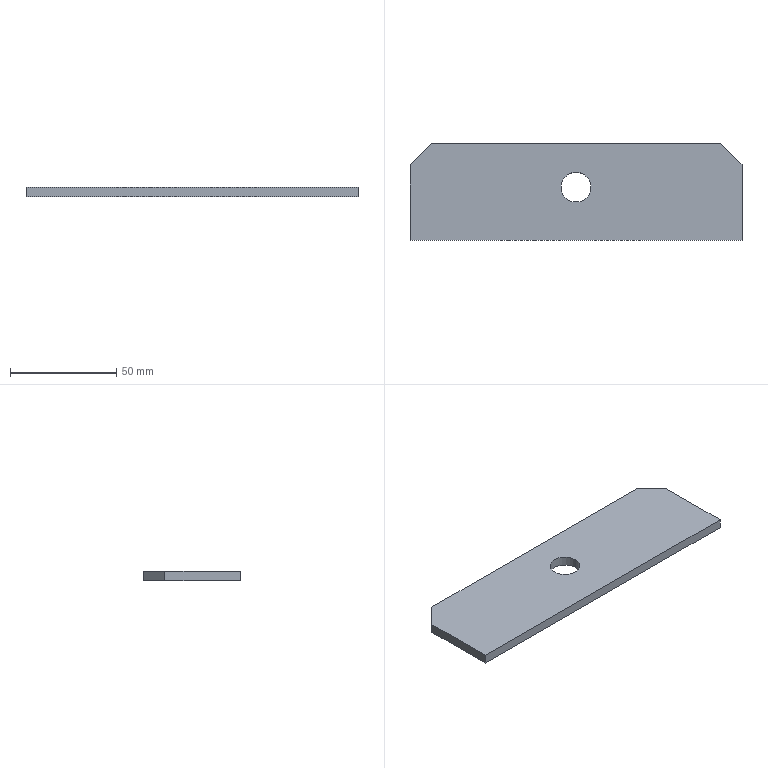Part | STEP file | DCV-000-014-B | 1 solid | 10 faces | box 156 x 45.5 x 4.5 mm | volume 30798 mm3 | plane 8 | cylinder 2 | commonest cylinder face diameters 14 x2
STEP:
#1=CARTESIAN_POINT('',(0.,0.,0.));
#2=DIRECTION('',(0.,0.,1.));
#3=DIRECTION('',(1.,0.,0.));
#4=AXIS2_PLACEMENT_3D('',#1,#2,#3);
#5=CARTESIAN_POINT('',(7.,25.,0.));
#6=VERTEX_POINT('',#5);
#7=CARTESIAN_POINT('',(7.,25.,4.5));
#8=VERTEX_POINT('',#7);
#9=CARTESIAN_POINT('',(7.,25.,-158.062));
#10=DIRECTION('',(0.,0.,1.));
#11=VECTOR('',#10,1.);
#12=LINE('',#9,#11);
#13=CARTESIAN_POINT('',(0.,25.,-158.062));
#14=DIRECTION('',(0.,0.,1.));
#15=DIRECTION('',(1.,0.,0.));
#16=AXIS2_PLACEMENT_3D('',#13,#14,#15);
#17=CYLINDRICAL_SURFACE('',#16,7.);
#18=CARTESIAN_POINT('',(6.283,0.));
#19=DIRECTION('',(0.,1.));
#20=VECTOR('',#19,1.);
#21=LINE('',#18,#20);
#22=(GEOMETRIC_REPRESENTATION_CONTEXT(2)PARAMETRIC_REPRESENTATION_CONTEXT()REPRESENTATION_CONTEXT('',''));
#23=DEFINITIONAL_REPRESENTATION('',(#21),#22);
#24=PCURVE('',#17,#23);
#25=CARTESIAN_POINT('',(0.,25.,-158.062));
#26=DIRECTION('',(0.,0.,1.));
#27=DIRECTION('',(1.,0.,0.));
#28=AXIS2_PLACEMENT_3D('',#25,#26,#27);
#29=CYLINDRICAL_SURFACE('',#28,7.);
#30=CARTESIAN_POINT('',(0.,0.));
#31=DIRECTION('',(0.,1.));
#32=VECTOR('',#31,1.);
#33=LINE('',#30,#32);
#34=(GEOMETRIC_REPRESENTATION_CONTEXT(2)PARAMETRIC_REPRESENTATION_CONTEXT()REPRESENTATION_CONTEXT('',''));
#35=DEFINITIONAL_REPRESENTATION('',(#33),#34);
#36=PCURVE('',#29,#35);
#37=SURFACE_CURVE('',#12,(#24,#36),.PCURVE_S1.);
#38=EDGE_CURVE('',#6,#8,#37,.T.);
#39=ORIENTED_EDGE('',*,*,#38,.T.);
#40=CARTESIAN_POINT('',(-7.,25.,4.5));
#41=VERTEX_POINT('',#40);
#42=CARTESIAN_POINT('',(0.,25.,4.5));
#43=DIRECTION('',(0.,0.,-1.));
#44=DIRECTION('',(1.,0.,0.));
#45=AXIS2_PLACEMENT_3D('',#42,#43,#44);
#46=CIRCLE('',#45,7.);
#47=CARTESIAN_POINT('',(6.283,162.562));
#48=DIRECTION('',(-1.,0.));
#49=VECTOR('',#48,1.);
#50=LINE('',#47,#49);
#51=(GEOMETRIC_REPRESENTATION_CONTEXT(2)PARAMETRIC_REPRESENTATION_CONTEXT()REPRESENTATION_CONTEXT('',''));
#52=DEFINITIONAL_REPRESENTATION('',(#50),#51);
#53=PCURVE('',#17,#52);
#54=CARTESIAN_POINT('',(0.,22.75,4.5));
#55=DIRECTION('',(0.,0.,1.));
#56=DIRECTION('',(1.,0.,0.));
#57=AXIS2_PLACEMENT_3D('',#54,#55,#56);
#58=PLANE('',#57);
#59=CARTESIAN_POINT('',(7.,2.25));
#60=CARTESIAN_POINT('',(7.,-9.874));
#61=CARTESIAN_POINT('',(-3.5,-3.812));
#62=CARTESIAN_POINT('',(-14.,2.25));
#63=CARTESIAN_POINT('',(-3.5,8.312));
#64=CARTESIAN_POINT('',(7.,14.374));
#65=CARTESIAN_POINT('',(7.,2.25));
#66=(BOUNDED_CURVE()B_SPLINE_CURVE(2,(#59,#60,#61,#62,#63,#64,#65),.UNSPECIFIED.,.T.,.F.)B_SPLINE_CURVE_WITH_KNOTS((1,2,2,2,2,1),(-2.094,0.,2.094,4.189,6.283,8.378),.UNSPECIFIED.)CURVE()GEOMETRIC_REPRESENTATION_ITEM()RATIONAL_B_SPLINE_CURVE((1.,0.5,1.,0.5,1.,0.5,1.))REPRESENTATION_ITEM(''));
#67=(GEOMETRIC_REPRESENTATION_CONTEXT(2)PARAMETRIC_REPRESENTATION_CONTEXT()REPRESENTATION_CONTEXT('',''));
#68=DEFINITIONAL_REPRESENTATION('',(#66),#67);
#69=PCURVE('',#58,#68);
#70=SURFACE_CURVE('',#46,(#53,#69),.PCURVE_S1.);
#71=EDGE_CURVE('',#8,#41,#70,.T.);
#72=ORIENTED_EDGE('',*,*,#71,.T.);
#73=CARTESIAN_POINT('',(-7.,25.,0.));
#74=VERTEX_POINT('',#73);
#75=CARTESIAN_POINT('',(-7.,25.,-158.062));
#76=DIRECTION('',(0.,0.,1.));
#77=VECTOR('',#76,1.);
#78=LINE('',#75,#77);
#79=CARTESIAN_POINT('',(3.142,0.));
#80=DIRECTION('',(0.,1.));
#81=VECTOR('',#80,1.);
#82=LINE('',#79,#81);
#83=(GEOMETRIC_REPRESENTATION_CONTEXT(2)PARAMETRIC_REPRESENTATION_CONTEXT()REPRESENTATION_CONTEXT('',''));
#84=DEFINITIONAL_REPRESENTATION('',(#82),#83);
#85=PCURVE('',#17,#84);
#86=CARTESIAN_POINT('',(3.142,0.));
#87=DIRECTION('',(0.,1.));
#88=VECTOR('',#87,1.);
#89=LINE('',#86,#88);
#90=(GEOMETRIC_REPRESENTATION_CONTEXT(2)PARAMETRIC_REPRESENTATION_CONTEXT()REPRESENTATION_CONTEXT('',''));
#91=DEFINITIONAL_REPRESENTATION('',(#89),#90);
#92=PCURVE('',#29,#91);
#93=SURFACE_CURVE('',#78,(#85,#92),.PCURVE_S1.);
#94=EDGE_CURVE('',#74,#41,#93,.T.);
#95=ORIENTED_EDGE('',*,*,#94,.F.);
#96=CARTESIAN_POINT('',(0.,25.,0.));
#97=DIRECTION('',(0.,0.,1.));
#98=DIRECTION('',(1.,0.,0.));
#99=AXIS2_PLACEMENT_3D('',#96,#97,#98);
#100=CIRCLE('',#99,7.);
#101=CARTESIAN_POINT('',(0.,158.062));
#102=DIRECTION('',(1.,0.));
#103=VECTOR('',#102,1.);
#104=LINE('',#101,#103);
#105=(GEOMETRIC_REPRESENTATION_CONTEXT(2)PARAMETRIC_REPRESENTATION_CONTEXT()REPRESENTATION_CONTEXT('',''));
#106=DEFINITIONAL_REPRESENTATION('',(#104),#105);
#107=PCURVE('',#17,#106);
#108=CARTESIAN_POINT('',(0.,22.75,0.));
#109=DIRECTION('',(0.,0.,1.));
#110=DIRECTION('',(1.,0.,0.));
#111=AXIS2_PLACEMENT_3D('',#108,#109,#110);
#112=PLANE('',#111);
#113=CARTESIAN_POINT('',(0.,2.25));
#114=DIRECTION('',(1.,0.));
#115=AXIS2_PLACEMENT_2D('',#113,#114);
#116=CIRCLE('',#115,7.);
#117=(GEOMETRIC_REPRESENTATION_CONTEXT(2)PARAMETRIC_REPRESENTATION_CONTEXT()REPRESENTATION_CONTEXT('',''));
#118=DEFINITIONAL_REPRESENTATION('',(#116),#117);
#119=PCURVE('',#112,#118);
#120=SURFACE_CURVE('',#100,(#107,#119),.PCURVE_S1.);
#121=EDGE_CURVE('',#74,#6,#120,.T.);
#122=ORIENTED_EDGE('',*,*,#121,.T.);
#123=EDGE_LOOP('',(#39,#72,#95,#122));
#124=FACE_BOUND('',#123,.F.);
#125=ADVANCED_FACE('',(#124),#17,.F.);
#126=CARTESIAN_POINT('',(0.,25.,0.));
#127=DIRECTION('',(0.,0.,1.));
#128=DIRECTION('',(1.,0.,0.));
#129=AXIS2_PLACEMENT_3D('',#126,#127,#128);
#130=CIRCLE('',#129,7.);
#131=CARTESIAN_POINT('',(0.,2.25));
#132=DIRECTION('',(1.,0.));
#133=AXIS2_PLACEMENT_2D('',#131,#132);
#134=CIRCLE('',#133,7.);
#135=(GEOMETRIC_REPRESENTATION_CONTEXT(2)PARAMETRIC_REPRESENTATION_CONTEXT()REPRESENTATION_CONTEXT('',''));
#136=DEFINITIONAL_REPRESENTATION('',(#134),#135);
#137=PCURVE('',#112,#136);
#138=CARTESIAN_POINT('',(0.,158.062));
#139=DIRECTION('',(1.,0.));
#140=VECTOR('',#139,1.);
#141=LINE('',#138,#140);
#142=(GEOMETRIC_REPRESENTATION_CONTEXT(2)PARAMETRIC_REPRESENTATION_CONTEXT()REPRESENTATION_CONTEXT('',''));
#143=DEFINITIONAL_REPRESENTATION('',(#141),#142);
#144=PCURVE('',#29,#143);
#145=SURFACE_CURVE('',#130,(#137,#144),.PCURVE_S1.);
#146=EDGE_CURVE('',#6,#74,#145,.T.);
#147=ORIENTED_EDGE('',*,*,#146,.T.);
#148=ORIENTED_EDGE('',*,*,#121,.T.);
#149=EDGE_LOOP('',(#147,#148));
#150=FACE_BOUND('',#149,.T.);
#151=CARTESIAN_POINT('',(78.,35.5,0.));
#152=VERTEX_POINT('',#151);
#153=CARTESIAN_POINT('',(68.,45.5,0.));
#154=VERTEX_POINT('',#153);
#155=CARTESIAN_POINT('',(59.188,54.312,0.));
#156=DIRECTION('',(-0.7071,0.7071,0.));
#157=VECTOR('',#156,1.);
#158=LINE('',#155,#157);
#159=CARTESIAN_POINT('',(59.188,31.563));
#160=DIRECTION('',(-0.7071,0.7071));
#161=VECTOR('',#160,1.);
#162=LINE('',#159,#161);
#163=(GEOMETRIC_REPRESENTATION_CONTEXT(2)PARAMETRIC_REPRESENTATION_CONTEXT()REPRESENTATION_CONTEXT('',''));
#164=DEFINITIONAL_REPRESENTATION('',(#162),#163);
#165=PCURVE('',#112,#164);
#166=CARTESIAN_POINT('',(73.,40.5,0.));
#167=DIRECTION('',(0.7071,0.7071,0.));
#168=DIRECTION('',(0.,0.,-1.));
#169=AXIS2_PLACEMENT_3D('',#166,#167,#168);
#170=PLANE('',#169);
#171=CARTESIAN_POINT('',(0.,19.534));
#172=DIRECTION('',(0.,1.));
#173=VECTOR('',#172,1.);
#174=LINE('',#171,#173);
#175=(GEOMETRIC_REPRESENTATION_CONTEXT(2)PARAMETRIC_REPRESENTATION_CONTEXT()REPRESENTATION_CONTEXT('',''));
#176=DEFINITIONAL_REPRESENTATION('',(#174),#175);
#177=PCURVE('',#170,#176);
#178=SURFACE_CURVE('',#158,(#165,#177),.PCURVE_S1.);
#179=EDGE_CURVE('',#152,#154,#178,.T.);
#180=ORIENTED_EDGE('',*,*,#179,.F.);
#181=CARTESIAN_POINT('',(78.,0.,0.));
#182=VERTEX_POINT('',#181);
#183=CARTESIAN_POINT('',(78.,0.,0.));
#184=DIRECTION('',(0.,1.,0.));
#185=VECTOR('',#184,1.);
#186=LINE('',#183,#185);
#187=CARTESIAN_POINT('',(78.,-22.75));
#188=DIRECTION('',(0.,1.));
#189=VECTOR('',#188,1.);
#190=LINE('',#187,#189);
#191=(GEOMETRIC_REPRESENTATION_CONTEXT(2)PARAMETRIC_REPRESENTATION_CONTEXT()REPRESENTATION_CONTEXT('',''));
#192=DEFINITIONAL_REPRESENTATION('',(#190),#191);
#193=PCURVE('',#112,#192);
#194=CARTESIAN_POINT('',(78.,0.,0.));
#195=DIRECTION('',(1.,0.,0.));
#196=DIRECTION('',(0.,-1.,0.));
#197=AXIS2_PLACEMENT_3D('',#194,#195,#196);
#198=PLANE('',#197);
#199=CARTESIAN_POINT('',(0.,0.));
#200=DIRECTION('',(-1.,0.));
#201=VECTOR('',#200,1.);
#202=LINE('',#199,#201);
#203=(GEOMETRIC_REPRESENTATION_CONTEXT(2)PARAMETRIC_REPRESENTATION_CONTEXT()REPRESENTATION_CONTEXT('',''));
#204=DEFINITIONAL_REPRESENTATION('',(#202),#203);
#205=PCURVE('',#198,#204);
#206=SURFACE_CURVE('',#186,(#193,#205),.PCURVE_S1.);
#207=EDGE_CURVE('',#182,#152,#206,.T.);
#208=ORIENTED_EDGE('',*,*,#207,.F.);
#209=CARTESIAN_POINT('',(-78.,0.,0.));
#210=VERTEX_POINT('',#209);
#211=CARTESIAN_POINT('',(-78.,0.,0.));
#212=DIRECTION('',(1.,0.,0.));
#213=VECTOR('',#212,1.);
#214=LINE('',#211,#213);
#215=CARTESIAN_POINT('',(-78.,-22.75));
#216=DIRECTION('',(1.,0.));
#217=VECTOR('',#216,1.);
#218=LINE('',#215,#217);
#219=(GEOMETRIC_REPRESENTATION_CONTEXT(2)PARAMETRIC_REPRESENTATION_CONTEXT()REPRESENTATION_CONTEXT('',''));
#220=DEFINITIONAL_REPRESENTATION('',(#218),#219);
#221=PCURVE('',#112,#220);
#222=CARTESIAN_POINT('',(-78.,0.,0.));
#223=DIRECTION('',(0.,-1.,0.));
#224=DIRECTION('',(0.,0.,-1.));
#225=AXIS2_PLACEMENT_3D('',#222,#223,#224);
#226=PLANE('',#225);
#227=CARTESIAN_POINT('',(0.,0.));
#228=DIRECTION('',(0.,1.));
#229=VECTOR('',#228,1.);
#230=LINE('',#227,#229);
#231=(GEOMETRIC_REPRESENTATION_CONTEXT(2)PARAMETRIC_REPRESENTATION_CONTEXT()REPRESENTATION_CONTEXT('',''));
#232=DEFINITIONAL_REPRESENTATION('',(#230),#231);
#233=PCURVE('',#226,#232);
#234=SURFACE_CURVE('',#214,(#221,#233),.PCURVE_S1.);
#235=EDGE_CURVE('',#210,#182,#234,.T.);
#236=ORIENTED_EDGE('',*,*,#235,.F.);
#237=CARTESIAN_POINT('',(-78.,35.5,0.));
#238=VERTEX_POINT('',#237);
#239=CARTESIAN_POINT('',(-78.,45.5,0.));
#240=DIRECTION('',(0.,-1.,0.));
#241=VECTOR('',#240,1.);
#242=LINE('',#239,#241);
#243=CARTESIAN_POINT('',(-78.,22.75));
#244=DIRECTION('',(0.,-1.));
#245=VECTOR('',#244,1.);
#246=LINE('',#243,#245);
#247=(GEOMETRIC_REPRESENTATION_CONTEXT(2)PARAMETRIC_REPRESENTATION_CONTEXT()REPRESENTATION_CONTEXT('',''));
#248=DEFINITIONAL_REPRESENTATION('',(#246),#247);
#249=PCURVE('',#112,#248);
#250=CARTESIAN_POINT('',(-78.,45.5,0.));
#251=DIRECTION('',(-1.,0.,0.));
#252=DIRECTION('',(0.,0.,1.));
#253=AXIS2_PLACEMENT_3D('',#250,#251,#252);
#254=PLANE('',#253);
#255=CARTESIAN_POINT('',(0.,0.));
#256=DIRECTION('',(0.,-1.));
#257=VECTOR('',#256,1.);
#258=LINE('',#255,#257);
#259=(GEOMETRIC_REPRESENTATION_CONTEXT(2)PARAMETRIC_REPRESENTATION_CONTEXT()REPRESENTATION_CONTEXT('',''));
#260=DEFINITIONAL_REPRESENTATION('',(#258),#259);
#261=PCURVE('',#254,#260);
#262=SURFACE_CURVE('',#242,(#249,#261),.PCURVE_S1.);
#263=EDGE_CURVE('',#238,#210,#262,.T.);
#264=ORIENTED_EDGE('',*,*,#263,.F.);
#265=CARTESIAN_POINT('',(-68.,45.5,0.));
#266=VERTEX_POINT('',#265);
#267=CARTESIAN_POINT('',(-59.188,54.312,0.));
#268=DIRECTION('',(-0.7071,-0.7071,0.));
#269=VECTOR('',#268,1.);
#270=LINE('',#267,#269);
#271=CARTESIAN_POINT('',(-59.188,31.563));
#272=DIRECTION('',(-0.7071,-0.7071));
#273=VECTOR('',#272,1.);
#274=LINE('',#271,#273);
#275=(GEOMETRIC_REPRESENTATION_CONTEXT(2)PARAMETRIC_REPRESENTATION_CONTEXT()REPRESENTATION_CONTEXT('',''));
#276=DEFINITIONAL_REPRESENTATION('',(#274),#275);
#277=PCURVE('',#112,#276);
#278=CARTESIAN_POINT('',(-73.,40.5,0.));
#279=DIRECTION('',(-0.7071,0.7071,0.));
#280=DIRECTION('',(0.,0.,1.));
#281=AXIS2_PLACEMENT_3D('',#278,#279,#280);
#282=PLANE('',#281);
#283=CARTESIAN_POINT('',(0.,19.534));
#284=DIRECTION('',(0.,-1.));
#285=VECTOR('',#284,1.);
#286=LINE('',#283,#285);
#287=(GEOMETRIC_REPRESENTATION_CONTEXT(2)PARAMETRIC_REPRESENTATION_CONTEXT()REPRESENTATION_CONTEXT('',''));
#288=DEFINITIONAL_REPRESENTATION('',(#286),#287);
#289=PCURVE('',#282,#288);
#290=SURFACE_CURVE('',#270,(#277,#289),.PCURVE_S1.);
#291=EDGE_CURVE('',#266,#238,#290,.T.);
#292=ORIENTED_EDGE('',*,*,#291,.F.);
#293=CARTESIAN_POINT('',(78.,45.5,0.));
#294=DIRECTION('',(-1.,0.,0.));
#295=VECTOR('',#294,1.);
#296=LINE('',#293,#295);
#297=CARTESIAN_POINT('',(78.,22.75));
#298=DIRECTION('',(-1.,0.));
#299=VECTOR('',#298,1.);
#300=LINE('',#297,#299);
#301=(GEOMETRIC_REPRESENTATION_CONTEXT(2)PARAMETRIC_REPRESENTATION_CONTEXT()REPRESENTATION_CONTEXT('',''));
#302=DEFINITIONAL_REPRESENTATION('',(#300),#301);
#303=PCURVE('',#112,#302);
#304=CARTESIAN_POINT('',(78.,45.5,0.));
#305=DIRECTION('',(0.,1.,0.));
#306=DIRECTION('',(1.,0.,0.));
#307=AXIS2_PLACEMENT_3D('',#304,#305,#306);
#308=PLANE('',#307);
#309=CARTESIAN_POINT('',(0.,0.));
#310=DIRECTION('',(-1.,0.));
#311=VECTOR('',#310,1.);
#312=LINE('',#309,#311);
#313=(GEOMETRIC_REPRESENTATION_CONTEXT(2)PARAMETRIC_REPRESENTATION_CONTEXT()REPRESENTATION_CONTEXT('',''));
#314=DEFINITIONAL_REPRESENTATION('',(#312),#313);
#315=PCURVE('',#308,#314);
#316=SURFACE_CURVE('',#296,(#303,#315),.PCURVE_S1.);
#317=EDGE_CURVE('',#154,#266,#316,.T.);
#318=ORIENTED_EDGE('',*,*,#317,.F.);
#319=EDGE_LOOP('',(#180,#208,#236,#264,#292,#318));
#320=FACE_BOUND('',#319,.T.);
#321=ADVANCED_FACE('',(#150,#320),#112,.F.);
#322=ORIENTED_EDGE('',*,*,#235,.T.);
#323=CARTESIAN_POINT('',(78.,0.,4.5));
#324=VERTEX_POINT('',#323);
#325=CARTESIAN_POINT('',(78.,0.,0.));
#326=DIRECTION('',(0.,0.,1.));
#327=VECTOR('',#326,1.);
#328=LINE('',#325,#327);
#329=CARTESIAN_POINT('',(0.,156.));
#330=DIRECTION('',(-1.,0.));
#331=VECTOR('',#330,1.);
#332=LINE('',#329,#331);
#333=(GEOMETRIC_REPRESENTATION_CONTEXT(2)PARAMETRIC_REPRESENTATION_CONTEXT()REPRESENTATION_CONTEXT('',''));
#334=DEFINITIONAL_REPRESENTATION('',(#332),#333);
#335=PCURVE('',#226,#334);
#336=CARTESIAN_POINT('',(0.,0.));
#337=DIRECTION('',(0.,-1.));
#338=VECTOR('',#337,1.);
#339=LINE('',#336,#338);
#340=(GEOMETRIC_REPRESENTATION_CONTEXT(2)PARAMETRIC_REPRESENTATION_CONTEXT()REPRESENTATION_CONTEXT('',''));
#341=DEFINITIONAL_REPRESENTATION('',(#339),#340);
#342=PCURVE('',#198,#341);
#343=SURFACE_CURVE('',#328,(#335,#342),.PCURVE_S1.);
#344=EDGE_CURVE('',#182,#324,#343,.T.);
#345=ORIENTED_EDGE('',*,*,#344,.T.);
#346=CARTESIAN_POINT('',(-78.,0.,4.5));
#347=VERTEX_POINT('',#346);
#348=CARTESIAN_POINT('',(-78.,0.,4.5));
#349=DIRECTION('',(1.,0.,0.));
#350=VECTOR('',#349,1.);
#351=LINE('',#348,#350);
#352=CARTESIAN_POINT('',(-4.5,0.));
#353=DIRECTION('',(0.,1.));
#354=VECTOR('',#353,1.);
#355=LINE('',#352,#354);
#356=(GEOMETRIC_REPRESENTATION_CONTEXT(2)PARAMETRIC_REPRESENTATION_CONTEXT()REPRESENTATION_CONTEXT('',''));
#357=DEFINITIONAL_REPRESENTATION('',(#355),#356);
#358=PCURVE('',#226,#357);
#359=CARTESIAN_POINT('',(-78.,-22.75));
#360=DIRECTION('',(1.,0.));
#361=VECTOR('',#360,1.);
#362=LINE('',#359,#361);
#363=(GEOMETRIC_REPRESENTATION_CONTEXT(2)PARAMETRIC_REPRESENTATION_CONTEXT()REPRESENTATION_CONTEXT('',''));
#364=DEFINITIONAL_REPRESENTATION('',(#362),#363);
#365=PCURVE('',#58,#364);
#366=SURFACE_CURVE('',#351,(#358,#365),.PCURVE_S1.);
#367=EDGE_CURVE('',#347,#324,#366,.T.);
#368=ORIENTED_EDGE('',*,*,#367,.F.);
#369=CARTESIAN_POINT('',(-78.,0.,0.));
#370=DIRECTION('',(0.,0.,1.));
#371=VECTOR('',#370,1.);
#372=LINE('',#369,#371);
#373=CARTESIAN_POINT('',(0.,0.));
#374=DIRECTION('',(-1.,0.));
#375=VECTOR('',#374,1.);
#376=LINE('',#373,#375);
#377=(GEOMETRIC_REPRESENTATION_CONTEXT(2)PARAMETRIC_REPRESENTATION_CONTEXT()REPRESENTATION_CONTEXT('',''));
#378=DEFINITIONAL_REPRESENTATION('',(#376),#377);
#379=PCURVE('',#226,#378);
#380=CARTESIAN_POINT('',(0.,-45.5));
#381=DIRECTION('',(1.,0.));
#382=VECTOR('',#381,1.);
#383=LINE('',#380,#382);
#384=(GEOMETRIC_REPRESENTATION_CONTEXT(2)PARAMETRIC_REPRESENTATION_CONTEXT()REPRESENTATION_CONTEXT('',''));
#385=DEFINITIONAL_REPRESENTATION('',(#383),#384);
#386=PCURVE('',#254,#385);
#387=SURFACE_CURVE('',#372,(#379,#386),.PCURVE_S1.);
#388=EDGE_CURVE('',#210,#347,#387,.T.);
#389=ORIENTED_EDGE('',*,*,#388,.F.);
#390=EDGE_LOOP('',(#322,#345,#368,#389));
#391=FACE_BOUND('',#390,.T.);
#392=ADVANCED_FACE('',(#391),#226,.T.);
#393=CARTESIAN_POINT('',(68.,45.5,4.5));
#394=VERTEX_POINT('',#393);
#395=CARTESIAN_POINT('',(68.,45.5,0.));
#396=DIRECTION('',(0.,0.,1.));
#397=VECTOR('',#396,1.);
#398=LINE('',#395,#397);
#399=CARTESIAN_POINT('',(-10.,0.));
#400=DIRECTION('',(0.,-1.));
#401=VECTOR('',#400,1.);
#402=LINE('',#399,#401);
#403=(GEOMETRIC_REPRESENTATION_CONTEXT(2)PARAMETRIC_REPRESENTATION_CONTEXT()REPRESENTATION_CONTEXT('',''));
#404=DEFINITIONAL_REPRESENTATION('',(#402),#403);
#405=PCURVE('',#308,#404);
#406=CARTESIAN_POINT('',(0.,7.071));
#407=DIRECTION('',(-1.,0.));
#408=VECTOR('',#407,1.);
#409=LINE('',#406,#408);
#410=(GEOMETRIC_REPRESENTATION_CONTEXT(2)PARAMETRIC_REPRESENTATION_CONTEXT()REPRESENTATION_CONTEXT('',''));
#411=DEFINITIONAL_REPRESENTATION('',(#409),#410);
#412=PCURVE('',#170,#411);
#413=SURFACE_CURVE('',#398,(#405,#412),.PCURVE_S1.);
#414=EDGE_CURVE('',#154,#394,#413,.T.);
#415=ORIENTED_EDGE('',*,*,#414,.F.);
#416=ORIENTED_EDGE('',*,*,#317,.T.);
#417=CARTESIAN_POINT('',(-68.,45.5,4.5));
#418=VERTEX_POINT('',#417);
#419=CARTESIAN_POINT('',(-68.,45.5,0.));
#420=DIRECTION('',(0.,0.,-1.));
#421=VECTOR('',#420,1.);
#422=LINE('',#419,#421);
#423=CARTESIAN_POINT('',(-146.,0.));
#424=DIRECTION('',(0.,1.));
#425=VECTOR('',#424,1.);
#426=LINE('',#423,#425);
#427=(GEOMETRIC_REPRESENTATION_CONTEXT(2)PARAMETRIC_REPRESENTATION_CONTEXT()REPRESENTATION_CONTEXT('',''));
#428=DEFINITIONAL_REPRESENTATION('',(#426),#427);
#429=PCURVE('',#308,#428);
#430=CARTESIAN_POINT('',(0.,7.071));
#431=DIRECTION('',(-1.,0.));
#432=VECTOR('',#431,1.);
#433=LINE('',#430,#432);
#434=(GEOMETRIC_REPRESENTATION_CONTEXT(2)PARAMETRIC_REPRESENTATION_CONTEXT()REPRESENTATION_CONTEXT('',''));
#435=DEFINITIONAL_REPRESENTATION('',(#433),#434);
#436=PCURVE('',#282,#435);
#437=SURFACE_CURVE('',#422,(#429,#436),.PCURVE_S1.);
#438=EDGE_CURVE('',#418,#266,#437,.T.);
#439=ORIENTED_EDGE('',*,*,#438,.F.);
#440=CARTESIAN_POINT('',(78.,45.5,4.5));
#441=DIRECTION('',(-1.,0.,0.));
#442=VECTOR('',#441,1.);
#443=LINE('',#440,#442);
#444=CARTESIAN_POINT('',(0.,-4.5));
#445=DIRECTION('',(-1.,0.));
#446=VECTOR('',#445,1.);
#447=LINE('',#444,#446);
#448=(GEOMETRIC_REPRESENTATION_CONTEXT(2)PARAMETRIC_REPRESENTATION_CONTEXT()REPRESENTATION_CONTEXT('',''));
#449=DEFINITIONAL_REPRESENTATION('',(#447),#448);
#450=PCURVE('',#308,#449);
#451=CARTESIAN_POINT('',(78.,22.75));
#452=DIRECTION('',(-1.,0.));
#453=VECTOR('',#452,1.);
#454=LINE('',#451,#453);
#455=(GEOMETRIC_REPRESENTATION_CONTEXT(2)PARAMETRIC_REPRESENTATION_CONTEXT()REPRESENTATION_CONTEXT('',''));
#456=DEFINITIONAL_REPRESENTATION('',(#454),#455);
#457=PCURVE('',#58,#456);
#458=SURFACE_CURVE('',#443,(#450,#457),.PCURVE_S1.);
#459=EDGE_CURVE('',#394,#418,#458,.T.);
#460=ORIENTED_EDGE('',*,*,#459,.F.);
#461=EDGE_LOOP('',(#415,#416,#439,#460));
#462=FACE_BOUND('',#461,.T.);
#463=ADVANCED_FACE('',(#462),#308,.T.);
#464=CARTESIAN_POINT('',(-78.,35.5,4.5));
#465=VERTEX_POINT('',#464);
#466=CARTESIAN_POINT('',(-78.,35.5,0.));
#467=DIRECTION('',(0.,0.,1.));
#468=VECTOR('',#467,1.);
#469=LINE('',#466,#468);
#470=CARTESIAN_POINT('',(0.,-10.));
#471=DIRECTION('',(1.,0.));
#472=VECTOR('',#471,1.);
#473=LINE('',#470,#472);
#474=(GEOMETRIC_REPRESENTATION_CONTEXT(2)PARAMETRIC_REPRESENTATION_CONTEXT()REPRESENTATION_CONTEXT('',''));
#475=DEFINITIONAL_REPRESENTATION('',(#473),#474);
#476=PCURVE('',#254,#475);
#477=CARTESIAN_POINT('',(0.,-7.071));
#478=DIRECTION('',(1.,0.));
#479=VECTOR('',#478,1.);
#480=LINE('',#477,#479);
#481=(GEOMETRIC_REPRESENTATION_CONTEXT(2)PARAMETRIC_REPRESENTATION_CONTEXT()REPRESENTATION_CONTEXT('',''));
#482=DEFINITIONAL_REPRESENTATION('',(#480),#481);
#483=PCURVE('',#282,#482);
#484=SURFACE_CURVE('',#469,(#476,#483),.PCURVE_S1.);
#485=EDGE_CURVE('',#238,#465,#484,.T.);
#486=ORIENTED_EDGE('',*,*,#485,.F.);
#487=ORIENTED_EDGE('',*,*,#263,.T.);
#488=ORIENTED_EDGE('',*,*,#388,.T.);
#489=CARTESIAN_POINT('',(-78.,45.5,4.5));
#490=DIRECTION('',(0.,-1.,0.));
#491=VECTOR('',#490,1.);
#492=LINE('',#489,#491);
#493=CARTESIAN_POINT('',(4.5,0.));
#494=DIRECTION('',(0.,-1.));
#495=VECTOR('',#494,1.);
#496=LINE('',#493,#495);
#497=(GEOMETRIC_REPRESENTATION_CONTEXT(2)PARAMETRIC_REPRESENTATION_CONTEXT()REPRESENTATION_CONTEXT('',''));
#498=DEFINITIONAL_REPRESENTATION('',(#496),#497);
#499=PCURVE('',#254,#498);
#500=CARTESIAN_POINT('',(-78.,22.75));
#501=DIRECTION('',(0.,-1.));
#502=VECTOR('',#501,1.);
#503=LINE('',#500,#502);
#504=(GEOMETRIC_REPRESENTATION_CONTEXT(2)PARAMETRIC_REPRESENTATION_CONTEXT()REPRESENTATION_CONTEXT('',''));
#505=DEFINITIONAL_REPRESENTATION('',(#503),#504);
#506=PCURVE('',#58,#505);
#507=SURFACE_CURVE('',#492,(#499,#506),.PCURVE_S1.);
#508=EDGE_CURVE('',#465,#347,#507,.T.);
#509=ORIENTED_EDGE('',*,*,#508,.F.);
#510=EDGE_LOOP('',(#486,#487,#488,#509));
#511=FACE_BOUND('',#510,.T.);
#512=ADVANCED_FACE('',(#511),#254,.T.);
#513=CARTESIAN_POINT('',(-59.188,54.312,4.5));
#514=DIRECTION('',(0.7071,0.7071,0.));
#515=VECTOR('',#514,1.);
#516=LINE('',#513,#515);
#517=CARTESIAN_POINT('',(4.5,19.534));
#518=DIRECTION('',(0.,1.));
#519=VECTOR('',#518,1.);
#520=LINE('',#517,#519);
#521=(GEOMETRIC_REPRESENTATION_CONTEXT(2)PARAMETRIC_REPRESENTATION_CONTEXT()REPRESENTATION_CONTEXT('',''));
#522=DEFINITIONAL_REPRESENTATION('',(#520),#521);
#523=PCURVE('',#282,#522);
#524=CARTESIAN_POINT('',(-59.188,31.563));
#525=DIRECTION('',(0.7071,0.7071));
#526=VECTOR('',#525,1.);
#527=LINE('',#524,#526);
#528=(GEOMETRIC_REPRESENTATION_CONTEXT(2)PARAMETRIC_REPRESENTATION_CONTEXT()REPRESENTATION_CONTEXT('',''));
#529=DEFINITIONAL_REPRESENTATION('',(#527),#528);
#530=PCURVE('',#58,#529);
#531=SURFACE_CURVE('',#516,(#523,#530),.PCURVE_S1.);
#532=EDGE_CURVE('',#465,#418,#531,.T.);
#533=ORIENTED_EDGE('',*,*,#532,.T.);
#534=ORIENTED_EDGE('',*,*,#438,.T.);
#535=ORIENTED_EDGE('',*,*,#291,.T.);
#536=ORIENTED_EDGE('',*,*,#485,.T.);
#537=EDGE_LOOP('',(#533,#534,#535,#536));
#538=FACE_BOUND('',#537,.T.);
#539=ADVANCED_FACE('',(#538),#282,.T.);
#540=ORIENTED_EDGE('',*,*,#71,.T.);
#541=CARTESIAN_POINT('',(0.,25.,4.5));
#542=DIRECTION('',(0.,0.,-1.));
#543=DIRECTION('',(1.,0.,0.));
#544=AXIS2_PLACEMENT_3D('',#541,#542,#543);
#545=CIRCLE('',#544,7.);
#546=CARTESIAN_POINT('',(7.,2.25));
#547=CARTESIAN_POINT('',(7.,-9.874));
#548=CARTESIAN_POINT('',(-3.5,-3.812));
#549=CARTESIAN_POINT('',(-14.,2.25));
#550=CARTESIAN_POINT('',(-3.5,8.312));
#551=CARTESIAN_POINT('',(7.,14.374));
#552=CARTESIAN_POINT('',(7.,2.25));
#553=(BOUNDED_CURVE()B_SPLINE_CURVE(2,(#546,#547,#548,#549,#550,#551,#552),.UNSPECIFIED.,.T.,.F.)B_SPLINE_CURVE_WITH_KNOTS((1,2,2,2,2,1),(-2.094,0.,2.094,4.189,6.283,8.378),.UNSPECIFIED.)CURVE()GEOMETRIC_REPRESENTATION_ITEM()RATIONAL_B_SPLINE_CURVE((1.,0.5,1.,0.5,1.,0.5,1.))REPRESENTATION_ITEM(''));
#554=(GEOMETRIC_REPRESENTATION_CONTEXT(2)PARAMETRIC_REPRESENTATION_CONTEXT()REPRESENTATION_CONTEXT('',''));
#555=DEFINITIONAL_REPRESENTATION('',(#553),#554);
#556=PCURVE('',#58,#555);
#557=CARTESIAN_POINT('',(6.283,162.562));
#558=DIRECTION('',(-1.,0.));
#559=VECTOR('',#558,1.);
#560=LINE('',#557,#559);
#561=(GEOMETRIC_REPRESENTATION_CONTEXT(2)PARAMETRIC_REPRESENTATION_CONTEXT()REPRESENTATION_CONTEXT('',''));
#562=DEFINITIONAL_REPRESENTATION('',(#560),#561);
#563=PCURVE('',#29,#562);
#564=SURFACE_CURVE('',#545,(#556,#563),.PCURVE_S1.);
#565=EDGE_CURVE('',#41,#8,#564,.T.);
#566=ORIENTED_EDGE('',*,*,#565,.T.);
#567=EDGE_LOOP('',(#540,#566));
#568=FACE_BOUND('',#567,.T.);
#569=CARTESIAN_POINT('',(78.,35.5,4.5));
#570=VERTEX_POINT('',#569);
#571=CARTESIAN_POINT('',(59.188,54.312,4.5));
#572=DIRECTION('',(0.7071,-0.7071,0.));
#573=VECTOR('',#572,1.);
#574=LINE('',#571,#573);
#575=CARTESIAN_POINT('',(59.188,31.563));
#576=DIRECTION('',(0.7071,-0.7071));
#577=VECTOR('',#576,1.);
#578=LINE('',#575,#577);
#579=(GEOMETRIC_REPRESENTATION_CONTEXT(2)PARAMETRIC_REPRESENTATION_CONTEXT()REPRESENTATION_CONTEXT('',''));
#580=DEFINITIONAL_REPRESENTATION('',(#578),#579);
#581=PCURVE('',#58,#580);
#582=CARTESIAN_POINT('',(-4.5,19.534));
#583=DIRECTION('',(0.,-1.));
#584=VECTOR('',#583,1.);
#585=LINE('',#582,#584);
#586=(GEOMETRIC_REPRESENTATION_CONTEXT(2)PARAMETRIC_REPRESENTATION_CONTEXT()REPRESENTATION_CONTEXT('',''));
#587=DEFINITIONAL_REPRESENTATION('',(#585),#586);
#588=PCURVE('',#170,#587);
#589=SURFACE_CURVE('',#574,(#581,#588),.PCURVE_S1.);
#590=EDGE_CURVE('',#394,#570,#589,.T.);
#591=ORIENTED_EDGE('',*,*,#590,.F.);
#592=ORIENTED_EDGE('',*,*,#459,.T.);
#593=ORIENTED_EDGE('',*,*,#532,.F.);
#594=ORIENTED_EDGE('',*,*,#508,.T.);
#595=ORIENTED_EDGE('',*,*,#367,.T.);
#596=CARTESIAN_POINT('',(78.,0.,4.5));
#597=DIRECTION('',(0.,1.,0.));
#598=VECTOR('',#597,1.);
#599=LINE('',#596,#598);
#600=CARTESIAN_POINT('',(78.,-22.75));
#601=DIRECTION('',(0.,1.));
#602=VECTOR('',#601,1.);
#603=LINE('',#600,#602);
#604=(GEOMETRIC_REPRESENTATION_CONTEXT(2)PARAMETRIC_REPRESENTATION_CONTEXT()REPRESENTATION_CONTEXT('',''));
#605=DEFINITIONAL_REPRESENTATION('',(#603),#604);
#606=PCURVE('',#58,#605);
#607=CARTESIAN_POINT('',(0.,-4.5));
#608=DIRECTION('',(-1.,0.));
#609=VECTOR('',#608,1.);
#610=LINE('',#607,#609);
#611=(GEOMETRIC_REPRESENTATION_CONTEXT(2)PARAMETRIC_REPRESENTATION_CONTEXT()REPRESENTATION_CONTEXT('',''));
#612=DEFINITIONAL_REPRESENTATION('',(#610),#611);
#613=PCURVE('',#198,#612);
#614=SURFACE_CURVE('',#599,(#606,#613),.PCURVE_S1.);
#615=EDGE_CURVE('',#324,#570,#614,.T.);
#616=ORIENTED_EDGE('',*,*,#615,.T.);
#617=EDGE_LOOP('',(#591,#592,#593,#594,#595,#616));
#618=FACE_BOUND('',#617,.T.);
#619=ADVANCED_FACE('',(#568,#618),#58,.T.);
#620=CARTESIAN_POINT('',(78.,35.5,0.));
#621=DIRECTION('',(0.,0.,-1.));
#622=VECTOR('',#621,1.);
#623=LINE('',#620,#622);
#624=CARTESIAN_POINT('',(-35.5,0.));
#625=DIRECTION('',(0.,1.));
#626=VECTOR('',#625,1.);
#627=LINE('',#624,#626);
#628=(GEOMETRIC_REPRESENTATION_CONTEXT(2)PARAMETRIC_REPRESENTATION_CONTEXT()REPRESENTATION_CONTEXT('',''));
#629=DEFINITIONAL_REPRESENTATION('',(#627),#628);
#630=PCURVE('',#198,#629);
#631=CARTESIAN_POINT('',(0.,-7.071));
#632=DIRECTION('',(1.,0.));
#633=VECTOR('',#632,1.);
#634=LINE('',#631,#633);
#635=(GEOMETRIC_REPRESENTATION_CONTEXT(2)PARAMETRIC_REPRESENTATION_CONTEXT()REPRESENTATION_CONTEXT('',''));
#636=DEFINITIONAL_REPRESENTATION('',(#634),#635);
#637=PCURVE('',#170,#636);
#638=SURFACE_CURVE('',#623,(#630,#637),.PCURVE_S1.);
#639=EDGE_CURVE('',#570,#152,#638,.T.);
#640=ORIENTED_EDGE('',*,*,#639,.F.);
#641=ORIENTED_EDGE('',*,*,#615,.F.);
#642=ORIENTED_EDGE('',*,*,#344,.F.);
#643=ORIENTED_EDGE('',*,*,#207,.T.);
#644=EDGE_LOOP('',(#640,#641,#642,#643));
#645=FACE_BOUND('',#644,.T.);
#646=ADVANCED_FACE('',(#645),#198,.T.);
#647=ORIENTED_EDGE('',*,*,#590,.T.);
#648=ORIENTED_EDGE('',*,*,#639,.T.);
#649=ORIENTED_EDGE('',*,*,#179,.T.);
#650=ORIENTED_EDGE('',*,*,#414,.T.);
#651=EDGE_LOOP('',(#647,#648,#649,#650));
#652=FACE_BOUND('',#651,.T.);
#653=ADVANCED_FACE('',(#652),#170,.T.);
#654=ORIENTED_EDGE('',*,*,#565,.T.);
#655=ORIENTED_EDGE('',*,*,#38,.F.);
#656=ORIENTED_EDGE('',*,*,#146,.T.);
#657=ORIENTED_EDGE('',*,*,#94,.T.);
#658=EDGE_LOOP('',(#654,#655,#656,#657));
#659=FACE_BOUND('',#658,.F.);
#660=ADVANCED_FACE('',(#659),#29,.F.);
#661=CLOSED_SHELL('',(#125,#321,#392,#463,#512,#539,#619,#646,#653,#660));
#662=MANIFOLD_SOLID_BREP('',#661);
#663=(LENGTH_UNIT()NAMED_UNIT(*)SI_UNIT(.MILLI.,.METRE.));
#664=UNCERTAINTY_MEASURE_WITH_UNIT(LENGTH_MEASURE(0.0000001),#663,'','');
#665=(NAMED_UNIT(*)PLANE_ANGLE_UNIT()SI_UNIT($,.RADIAN.));
#666=(NAMED_UNIT(*)SI_UNIT($,.STERADIAN.)SOLID_ANGLE_UNIT());
#667=(GEOMETRIC_REPRESENTATION_CONTEXT(3)GLOBAL_UNCERTAINTY_ASSIGNED_CONTEXT((#664))GLOBAL_UNIT_ASSIGNED_CONTEXT((#663,#665,#666))REPRESENTATION_CONTEXT('',''));
#668=ADVANCED_BREP_SHAPE_REPRESENTATION('',(#4,#662),#667);